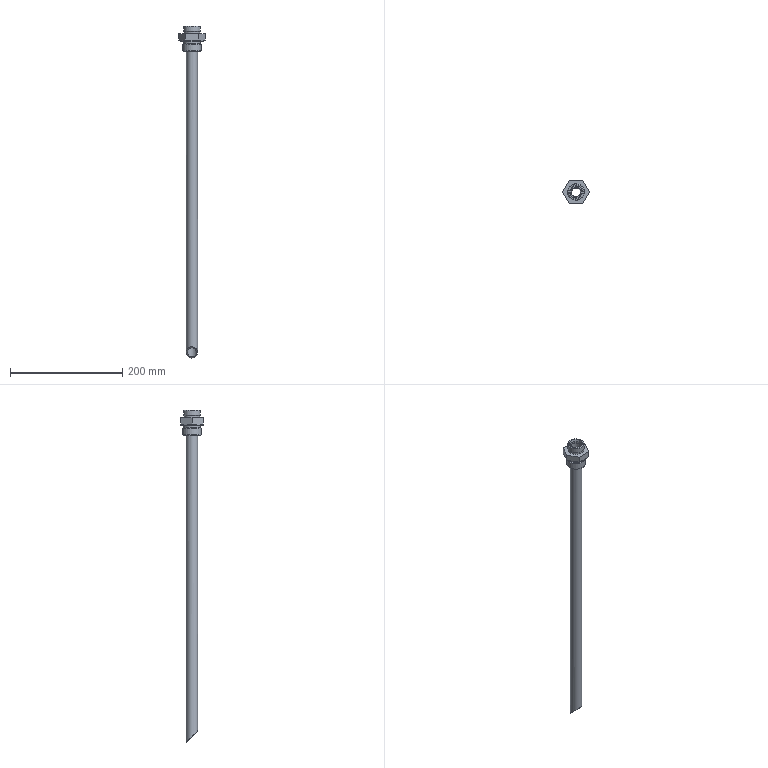Part | STEP file | HL4GZ-1.581.019 (radiator return pipe weldment) | 2 solids | 40 faces | box 47.343 x 41 x 592 mm | volume 83507 mm3 | plane 23 | cylinder 11 | cone 6 | commonest cylinder face diameters 30 x2 16.4 x1 19 x1 20 x1 21.5 x1 22 x1